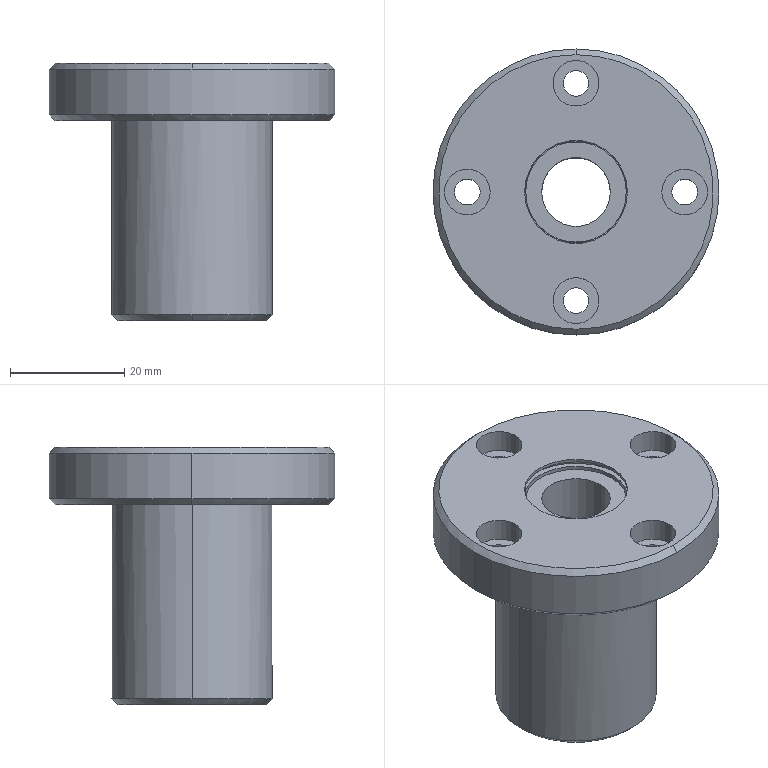Part | STEP file | fBY02F02M-00-30A | 2 solids | 56 faces | box 50 x 50 x 45 mm | volume 36506 mm3 | cylinder 36 | plane 14 | cone 6 | commonest cylinder face diameters 4.5 x8 8 x8 12 x4 17.6 x4 18 x4 12.5 x2